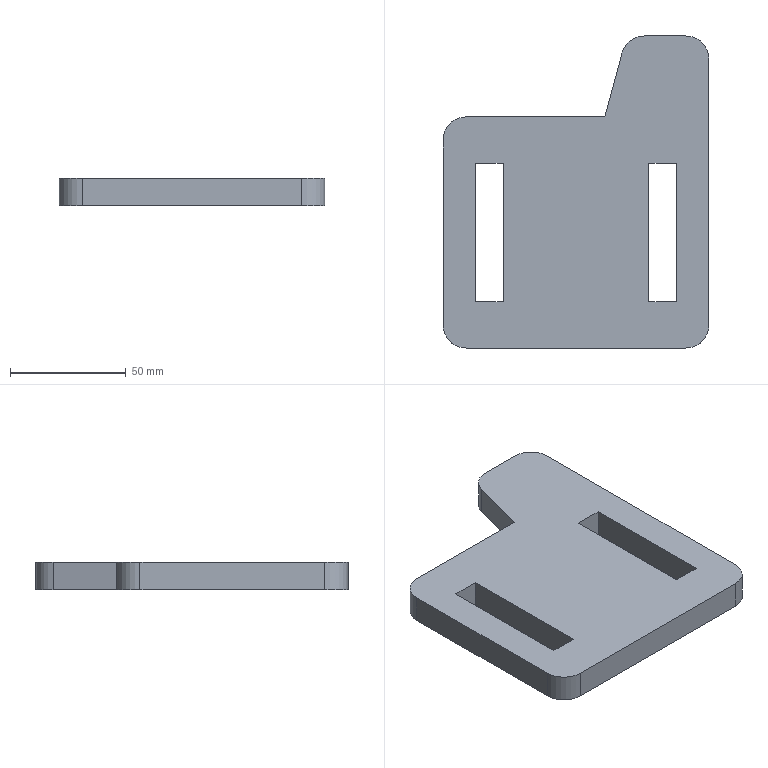Part | SolidWorks | features FlatPattern 1, SMBaseFlange 1, SheetMetal 1 | 1 solid | 21 faces | box 115 x 135 x 12 mm | volume 136485 mm3 | plane 16 | cylinder 5 | commonest cylinder face diameters 20 x5
STEP:
#1=CARTESIAN_POINT('',(3.778,-205.509,0.));
#2=VERTEX_POINT('',#1);
#3=CARTESIAN_POINT('',(-56.222,-205.509,0.));
#4=VERTEX_POINT('',#3);
#5=CARTESIAN_POINT('',(3.778,-205.509,0.));
#6=DIRECTION('',(-1.,0.,0.));
#7=VECTOR('',#6,1000.);
#8=LINE('',#5,#7);
#9=EDGE_CURVE('',#2,#4,#8,.T.);
#10=ORIENTED_EDGE('',*,*,#9,.F.);
#11=CARTESIAN_POINT('',(3.778,-205.509,-12.));
#12=VERTEX_POINT('',#11);
#13=CARTESIAN_POINT('',(3.778,-205.509,-12.));
#14=DIRECTION('',(0.,0.,1.));
#15=VECTOR('',#14,1000.);
#16=LINE('',#13,#15);
#17=EDGE_CURVE('',#12,#2,#16,.T.);
#18=ORIENTED_EDGE('',*,*,#17,.F.);
#19=CARTESIAN_POINT('',(-56.222,-205.509,-12.));
#20=VERTEX_POINT('',#19);
#21=CARTESIAN_POINT('',(3.778,-205.509,-12.));
#22=DIRECTION('',(-1.,0.,0.));
#23=VECTOR('',#22,1000.);
#24=LINE('',#21,#23);
#25=EDGE_CURVE('',#12,#20,#24,.T.);
#26=ORIENTED_EDGE('',*,*,#25,.T.);
#27=CARTESIAN_POINT('',(-56.222,-205.509,-12.));
#28=DIRECTION('',(0.,0.,1.));
#29=VECTOR('',#28,1000.);
#30=LINE('',#27,#29);
#31=EDGE_CURVE('',#20,#4,#30,.T.);
#32=ORIENTED_EDGE('',*,*,#31,.T.);
#33=EDGE_LOOP('',(#10,#18,#26,#32));
#34=FACE_OUTER_BOUND('',#33,.T.);
#35=CARTESIAN_POINT('',(3.778,-205.509,-12.));
#36=DIRECTION('',(0.,1.,0.));
#37=DIRECTION('',(0.,0.,1.));
#38=AXIS2_PLACEMENT_3D('',#35,#36,#37);
#39=PLANE('',#38);
#40=ADVANCED_FACE('',(#34),#39,.T.);
#41=CARTESIAN_POINT('',(11.17,-177.921,0.));
#42=VERTEX_POINT('',#41);
#43=CARTESIAN_POINT('',(11.17,-177.921,0.));
#44=DIRECTION('',(-0.2588,-0.9659,0.));
#45=VECTOR('',#44,1000.);
#46=LINE('',#43,#45);
#47=EDGE_CURVE('',#42,#2,#46,.T.);
#48=ORIENTED_EDGE('',*,*,#47,.F.);
#49=CARTESIAN_POINT('',(11.17,-177.921,-12.));
#50=VERTEX_POINT('',#49);
#51=CARTESIAN_POINT('',(11.17,-177.921,-12.));
#52=DIRECTION('',(0.,0.,1.));
#53=VECTOR('',#52,1000.);
#54=LINE('',#51,#53);
#55=EDGE_CURVE('',#50,#42,#54,.T.);
#56=ORIENTED_EDGE('',*,*,#55,.F.);
#57=CARTESIAN_POINT('',(11.17,-177.921,-12.));
#58=DIRECTION('',(-0.2588,-0.9659,0.));
#59=VECTOR('',#58,1000.);
#60=LINE('',#57,#59);
#61=EDGE_CURVE('',#50,#12,#60,.T.);
#62=ORIENTED_EDGE('',*,*,#61,.T.);
#63=ORIENTED_EDGE('',*,*,#17,.T.);
#64=EDGE_LOOP('',(#48,#56,#62,#63));
#65=FACE_OUTER_BOUND('',#64,.T.);
#66=CARTESIAN_POINT('',(11.17,-177.921,-12.));
#67=DIRECTION('',(-0.9659,0.2588,0.));
#68=DIRECTION('',(-0.2588,-0.9659,0.));
#69=AXIS2_PLACEMENT_3D('',#66,#67,#68);
#70=PLANE('',#69);
#71=ADVANCED_FACE('',(#65),#70,.T.);
#72=CARTESIAN_POINT('',(20.829,-170.509,0.));
#73=VERTEX_POINT('',#72);
#74=CARTESIAN_POINT('',(20.829,-180.509,0.));
#75=DIRECTION('',(0.,0.,1.));
#76=DIRECTION('',(1.,0.,0.));
#77=AXIS2_PLACEMENT_3D('',#74,#75,#76);
#78=CIRCLE('',#77,10.);
#79=EDGE_CURVE('',#73,#42,#78,.T.);
#80=ORIENTED_EDGE('',*,*,#79,.F.);
#81=CARTESIAN_POINT('',(20.829,-170.509,-12.));
#82=VERTEX_POINT('',#81);
#83=CARTESIAN_POINT('',(20.829,-170.509,-12.));
#84=DIRECTION('',(0.,0.,1.));
#85=VECTOR('',#84,1000.);
#86=LINE('',#83,#85);
#87=EDGE_CURVE('',#82,#73,#86,.T.);
#88=ORIENTED_EDGE('',*,*,#87,.F.);
#89=CARTESIAN_POINT('',(20.829,-180.509,-12.));
#90=DIRECTION('',(0.,0.,1.));
#91=DIRECTION('',(1.,0.,0.));
#92=AXIS2_PLACEMENT_3D('',#89,#90,#91);
#93=CIRCLE('',#92,10.);
#94=EDGE_CURVE('',#82,#50,#93,.T.);
#95=ORIENTED_EDGE('',*,*,#94,.T.);
#96=ORIENTED_EDGE('',*,*,#55,.T.);
#97=EDGE_LOOP('',(#80,#88,#95,#96));
#98=FACE_OUTER_BOUND('',#97,.T.);
#99=CARTESIAN_POINT('',(20.829,-180.509,-12.));
#100=DIRECTION('',(0.,0.,1.));
#101=DIRECTION('',(1.,0.,0.));
#102=AXIS2_PLACEMENT_3D('',#99,#100,#101);
#103=CYLINDRICAL_SURFACE('',#102,10.);
#104=ADVANCED_FACE('',(#98),#103,.T.);
#105=CARTESIAN_POINT('',(38.778,-170.509,0.));
#106=VERTEX_POINT('',#105);
#107=CARTESIAN_POINT('',(20.829,-170.509,0.));
#108=DIRECTION('',(-1.,0.,0.));
#109=VECTOR('',#108,1000.);
#110=LINE('',#107,#109);
#111=EDGE_CURVE('',#106,#73,#110,.T.);
#112=ORIENTED_EDGE('',*,*,#111,.F.);
#113=CARTESIAN_POINT('',(38.778,-170.509,-12.));
#114=VERTEX_POINT('',#113);
#115=CARTESIAN_POINT('',(38.778,-170.509,-12.));
#116=DIRECTION('',(0.,0.,1.));
#117=VECTOR('',#116,1000.);
#118=LINE('',#115,#117);
#119=EDGE_CURVE('',#114,#106,#118,.T.);
#120=ORIENTED_EDGE('',*,*,#119,.F.);
#121=CARTESIAN_POINT('',(20.829,-170.509,-12.));
#122=DIRECTION('',(-1.,0.,0.));
#123=VECTOR('',#122,1000.);
#124=LINE('',#121,#123);
#125=EDGE_CURVE('',#114,#82,#124,.T.);
#126=ORIENTED_EDGE('',*,*,#125,.T.);
#127=ORIENTED_EDGE('',*,*,#87,.T.);
#128=EDGE_LOOP('',(#112,#120,#126,#127));
#129=FACE_OUTER_BOUND('',#128,.T.);
#130=CARTESIAN_POINT('',(20.829,-170.509,-12.));
#131=DIRECTION('',(0.,1.,0.));
#132=DIRECTION('',(-1.,0.,0.));
#133=AXIS2_PLACEMENT_3D('',#130,#131,#132);
#134=PLANE('',#133);
#135=ADVANCED_FACE('',(#129),#134,.T.);
#136=CARTESIAN_POINT('',(48.778,-180.509,0.));
#137=VERTEX_POINT('',#136);
#138=CARTESIAN_POINT('',(38.778,-180.509,0.));
#139=DIRECTION('',(0.,0.,1.));
#140=DIRECTION('',(-1.,0.,0.));
#141=AXIS2_PLACEMENT_3D('',#138,#139,#140);
#142=CIRCLE('',#141,10.);
#143=EDGE_CURVE('',#137,#106,#142,.T.);
#144=ORIENTED_EDGE('',*,*,#143,.F.);
#145=CARTESIAN_POINT('',(48.778,-180.509,-12.));
#146=VERTEX_POINT('',#145);
#147=CARTESIAN_POINT('',(48.778,-180.509,-12.));
#148=DIRECTION('',(0.,0.,1.));
#149=VECTOR('',#148,1000.);
#150=LINE('',#147,#149);
#151=EDGE_CURVE('',#146,#137,#150,.T.);
#152=ORIENTED_EDGE('',*,*,#151,.F.);
#153=CARTESIAN_POINT('',(38.778,-180.509,-12.));
#154=DIRECTION('',(0.,0.,1.));
#155=DIRECTION('',(-1.,0.,0.));
#156=AXIS2_PLACEMENT_3D('',#153,#154,#155);
#157=CIRCLE('',#156,10.);
#158=EDGE_CURVE('',#146,#114,#157,.T.);
#159=ORIENTED_EDGE('',*,*,#158,.T.);
#160=ORIENTED_EDGE('',*,*,#119,.T.);
#161=EDGE_LOOP('',(#144,#152,#159,#160));
#162=FACE_OUTER_BOUND('',#161,.T.);
#163=CARTESIAN_POINT('',(38.778,-180.509,-12.));
#164=DIRECTION('',(0.,0.,1.));
#165=DIRECTION('',(1.,0.,0.));
#166=AXIS2_PLACEMENT_3D('',#163,#164,#165);
#167=CYLINDRICAL_SURFACE('',#166,10.);
#168=ADVANCED_FACE('',(#162),#167,.T.);
#169=CARTESIAN_POINT('',(48.778,-295.509,0.));
#170=VERTEX_POINT('',#169);
#171=CARTESIAN_POINT('',(48.778,-180.509,0.));
#172=DIRECTION('',(0.,1.,0.));
#173=VECTOR('',#172,1000.);
#174=LINE('',#171,#173);
#175=EDGE_CURVE('',#170,#137,#174,.T.);
#176=ORIENTED_EDGE('',*,*,#175,.F.);
#177=CARTESIAN_POINT('',(48.778,-295.509,-12.));
#178=VERTEX_POINT('',#177);
#179=CARTESIAN_POINT('',(48.778,-295.509,-12.));
#180=DIRECTION('',(0.,0.,1.));
#181=VECTOR('',#180,1000.);
#182=LINE('',#179,#181);
#183=EDGE_CURVE('',#178,#170,#182,.T.);
#184=ORIENTED_EDGE('',*,*,#183,.F.);
#185=CARTESIAN_POINT('',(48.778,-180.509,-12.));
#186=DIRECTION('',(0.,1.,0.));
#187=VECTOR('',#186,1000.);
#188=LINE('',#185,#187);
#189=EDGE_CURVE('',#178,#146,#188,.T.);
#190=ORIENTED_EDGE('',*,*,#189,.T.);
#191=ORIENTED_EDGE('',*,*,#151,.T.);
#192=EDGE_LOOP('',(#176,#184,#190,#191));
#193=FACE_OUTER_BOUND('',#192,.T.);
#194=CARTESIAN_POINT('',(48.778,-180.509,-12.));
#195=DIRECTION('',(1.,0.,0.));
#196=DIRECTION('',(0.,1.,0.));
#197=AXIS2_PLACEMENT_3D('',#194,#195,#196);
#198=PLANE('',#197);
#199=ADVANCED_FACE('',(#193),#198,.T.);
#200=CARTESIAN_POINT('',(38.778,-305.509,0.));
#201=VERTEX_POINT('',#200);
#202=CARTESIAN_POINT('',(38.778,-295.509,0.));
#203=DIRECTION('',(0.,0.,1.));
#204=DIRECTION('',(-1.,0.,0.));
#205=AXIS2_PLACEMENT_3D('',#202,#203,#204);
#206=CIRCLE('',#205,10.);
#207=EDGE_CURVE('',#201,#170,#206,.T.);
#208=ORIENTED_EDGE('',*,*,#207,.F.);
#209=CARTESIAN_POINT('',(38.778,-305.509,-12.));
#210=VERTEX_POINT('',#209);
#211=CARTESIAN_POINT('',(38.778,-305.509,-12.));
#212=DIRECTION('',(0.,0.,1.));
#213=VECTOR('',#212,1000.);
#214=LINE('',#211,#213);
#215=EDGE_CURVE('',#210,#201,#214,.T.);
#216=ORIENTED_EDGE('',*,*,#215,.F.);
#217=CARTESIAN_POINT('',(38.778,-295.509,-12.));
#218=DIRECTION('',(0.,0.,1.));
#219=DIRECTION('',(-1.,0.,0.));
#220=AXIS2_PLACEMENT_3D('',#217,#218,#219);
#221=CIRCLE('',#220,10.);
#222=EDGE_CURVE('',#210,#178,#221,.T.);
#223=ORIENTED_EDGE('',*,*,#222,.T.);
#224=ORIENTED_EDGE('',*,*,#183,.T.);
#225=EDGE_LOOP('',(#208,#216,#223,#224));
#226=FACE_OUTER_BOUND('',#225,.T.);
#227=CARTESIAN_POINT('',(38.778,-295.509,-12.));
#228=DIRECTION('',(0.,0.,1.));
#229=DIRECTION('',(1.,0.,0.));
#230=AXIS2_PLACEMENT_3D('',#227,#228,#229);
#231=CYLINDRICAL_SURFACE('',#230,10.);
#232=ADVANCED_FACE('',(#226),#231,.T.);
#233=CARTESIAN_POINT('',(-56.222,-305.509,0.));
#234=VERTEX_POINT('',#233);
#235=CARTESIAN_POINT('',(-56.222,-305.509,0.));
#236=DIRECTION('',(1.,0.,0.));
#237=VECTOR('',#236,1000.);
#238=LINE('',#235,#237);
#239=EDGE_CURVE('',#234,#201,#238,.T.);
#240=ORIENTED_EDGE('',*,*,#239,.F.);
#241=CARTESIAN_POINT('',(-56.222,-305.509,-12.));
#242=VERTEX_POINT('',#241);
#243=CARTESIAN_POINT('',(-56.222,-305.509,-12.));
#244=DIRECTION('',(0.,0.,1.));
#245=VECTOR('',#244,1000.);
#246=LINE('',#243,#245);
#247=EDGE_CURVE('',#242,#234,#246,.T.);
#248=ORIENTED_EDGE('',*,*,#247,.F.);
#249=CARTESIAN_POINT('',(-56.222,-305.509,-12.));
#250=DIRECTION('',(1.,0.,0.));
#251=VECTOR('',#250,1000.);
#252=LINE('',#249,#251);
#253=EDGE_CURVE('',#242,#210,#252,.T.);
#254=ORIENTED_EDGE('',*,*,#253,.T.);
#255=ORIENTED_EDGE('',*,*,#215,.T.);
#256=EDGE_LOOP('',(#240,#248,#254,#255));
#257=FACE_OUTER_BOUND('',#256,.T.);
#258=CARTESIAN_POINT('',(-56.222,-305.509,-12.));
#259=DIRECTION('',(0.,-1.,0.));
#260=DIRECTION('',(0.,0.,-1.));
#261=AXIS2_PLACEMENT_3D('',#258,#259,#260);
#262=PLANE('',#261);
#263=ADVANCED_FACE('',(#257),#262,.T.);
#264=CARTESIAN_POINT('',(-66.222,-295.509,0.));
#265=VERTEX_POINT('',#264);
#266=CARTESIAN_POINT('',(-56.222,-295.509,0.));
#267=DIRECTION('',(0.,0.,1.));
#268=DIRECTION('',(1.,0.,0.));
#269=AXIS2_PLACEMENT_3D('',#266,#267,#268);
#270=CIRCLE('',#269,10.);
#271=EDGE_CURVE('',#265,#234,#270,.T.);
#272=ORIENTED_EDGE('',*,*,#271,.F.);
#273=CARTESIAN_POINT('',(-66.222,-295.509,-12.));
#274=VERTEX_POINT('',#273);
#275=CARTESIAN_POINT('',(-66.222,-295.509,-12.));
#276=DIRECTION('',(0.,0.,1.));
#277=VECTOR('',#276,1000.);
#278=LINE('',#275,#277);
#279=EDGE_CURVE('',#274,#265,#278,.T.);
#280=ORIENTED_EDGE('',*,*,#279,.F.);
#281=CARTESIAN_POINT('',(-56.222,-295.509,-12.));
#282=DIRECTION('',(0.,0.,1.));
#283=DIRECTION('',(1.,0.,0.));
#284=AXIS2_PLACEMENT_3D('',#281,#282,#283);
#285=CIRCLE('',#284,10.);
#286=EDGE_CURVE('',#274,#242,#285,.T.);
#287=ORIENTED_EDGE('',*,*,#286,.T.);
#288=ORIENTED_EDGE('',*,*,#247,.T.);
#289=EDGE_LOOP('',(#272,#280,#287,#288));
#290=FACE_OUTER_BOUND('',#289,.T.);
#291=CARTESIAN_POINT('',(-56.222,-295.509,-12.));
#292=DIRECTION('',(0.,0.,1.));
#293=DIRECTION('',(1.,0.,0.));
#294=AXIS2_PLACEMENT_3D('',#291,#292,#293);
#295=CYLINDRICAL_SURFACE('',#294,10.);
#296=ADVANCED_FACE('',(#290),#295,.T.);
#297=CARTESIAN_POINT('',(-66.222,-215.509,0.));
#298=VERTEX_POINT('',#297);
#299=CARTESIAN_POINT('',(-66.222,-215.509,0.));
#300=DIRECTION('',(0.,-1.,0.));
#301=VECTOR('',#300,1000.);
#302=LINE('',#299,#301);
#303=EDGE_CURVE('',#298,#265,#302,.T.);
#304=ORIENTED_EDGE('',*,*,#303,.F.);
#305=CARTESIAN_POINT('',(-66.222,-215.509,-12.));
#306=VERTEX_POINT('',#305);
#307=CARTESIAN_POINT('',(-66.222,-215.509,-12.));
#308=DIRECTION('',(0.,0.,1.));
#309=VECTOR('',#308,1000.);
#310=LINE('',#307,#309);
#311=EDGE_CURVE('',#306,#298,#310,.T.);
#312=ORIENTED_EDGE('',*,*,#311,.F.);
#313=CARTESIAN_POINT('',(-66.222,-215.509,-12.));
#314=DIRECTION('',(0.,-1.,0.));
#315=VECTOR('',#314,1000.);
#316=LINE('',#313,#315);
#317=EDGE_CURVE('',#306,#274,#316,.T.);
#318=ORIENTED_EDGE('',*,*,#317,.T.);
#319=ORIENTED_EDGE('',*,*,#279,.T.);
#320=EDGE_LOOP('',(#304,#312,#318,#319));
#321=FACE_OUTER_BOUND('',#320,.T.);
#322=CARTESIAN_POINT('',(-66.222,-215.509,-12.));
#323=DIRECTION('',(-1.,0.,0.));
#324=DIRECTION('',(0.,-1.,0.));
#325=AXIS2_PLACEMENT_3D('',#322,#323,#324);
#326=PLANE('',#325);
#327=ADVANCED_FACE('',(#321),#326,.T.);
#328=CARTESIAN_POINT('',(-56.222,-215.509,0.));
#329=DIRECTION('',(0.,0.,1.));
#330=DIRECTION('',(1.,0.,0.));
#331=AXIS2_PLACEMENT_3D('',#328,#329,#330);
#332=CIRCLE('',#331,10.);
#333=EDGE_CURVE('',#4,#298,#332,.T.);
#334=ORIENTED_EDGE('',*,*,#333,.F.);
#335=ORIENTED_EDGE('',*,*,#31,.F.);
#336=CARTESIAN_POINT('',(-56.222,-215.509,-12.));
#337=DIRECTION('',(0.,0.,1.));
#338=DIRECTION('',(1.,0.,0.));
#339=AXIS2_PLACEMENT_3D('',#336,#337,#338);
#340=CIRCLE('',#339,10.);
#341=EDGE_CURVE('',#20,#306,#340,.T.);
#342=ORIENTED_EDGE('',*,*,#341,.T.);
#343=ORIENTED_EDGE('',*,*,#311,.T.);
#344=EDGE_LOOP('',(#334,#335,#342,#343));
#345=FACE_OUTER_BOUND('',#344,.T.);
#346=CARTESIAN_POINT('',(-56.222,-215.509,-12.));
#347=DIRECTION('',(0.,0.,1.));
#348=DIRECTION('',(1.,0.,0.));
#349=AXIS2_PLACEMENT_3D('',#346,#347,#348);
#350=CYLINDRICAL_SURFACE('',#349,10.);
#351=ADVANCED_FACE('',(#345),#350,.T.);
#352=CARTESIAN_POINT('',(-40.222,-225.509,-12.));
#353=VERTEX_POINT('',#352);
#354=CARTESIAN_POINT('',(-52.222,-225.509,-12.));
#355=VERTEX_POINT('',#354);
#356=CARTESIAN_POINT('',(-52.222,-225.509,-12.));
#357=DIRECTION('',(-1.,0.,0.));
#358=VECTOR('',#357,1000.);
#359=LINE('',#356,#358);
#360=EDGE_CURVE('',#353,#355,#359,.T.);
#361=ORIENTED_EDGE('',*,*,#360,.T.);
#362=CARTESIAN_POINT('',(-52.222,-285.509,-12.));
#363=VERTEX_POINT('',#362);
#364=CARTESIAN_POINT('',(-52.222,-225.509,-12.));
#365=DIRECTION('',(0.,-1.,0.));
#366=VECTOR('',#365,1000.);
#367=LINE('',#364,#366);
#368=EDGE_CURVE('',#355,#363,#367,.T.);
#369=ORIENTED_EDGE('',*,*,#368,.T.);
#370=CARTESIAN_POINT('',(-40.222,-285.509,-12.));
#371=VERTEX_POINT('',#370);
#372=CARTESIAN_POINT('',(-52.222,-285.509,-12.));
#373=DIRECTION('',(1.,0.,0.));
#374=VECTOR('',#373,1000.);
#375=LINE('',#372,#374);
#376=EDGE_CURVE('',#363,#371,#375,.T.);
#377=ORIENTED_EDGE('',*,*,#376,.T.);
#378=CARTESIAN_POINT('',(-40.222,-225.509,-12.));
#379=DIRECTION('',(0.,1.,0.));
#380=VECTOR('',#379,1000.);
#381=LINE('',#378,#380);
#382=EDGE_CURVE('',#371,#353,#381,.T.);
#383=ORIENTED_EDGE('',*,*,#382,.T.);
#384=EDGE_LOOP('',(#361,#369,#377,#383));
#385=FACE_BOUND('',#384,.T.);
#386=CARTESIAN_POINT('',(34.778,-225.509,-12.));
#387=VERTEX_POINT('',#386);
#388=CARTESIAN_POINT('',(22.778,-225.509,-12.));
#389=VERTEX_POINT('',#388);
#390=CARTESIAN_POINT('',(22.778,-225.509,-12.));
#391=DIRECTION('',(-1.,0.,0.));
#392=VECTOR('',#391,1000.);
#393=LINE('',#390,#392);
#394=EDGE_CURVE('',#387,#389,#393,.T.);
#395=ORIENTED_EDGE('',*,*,#394,.T.);
#396=CARTESIAN_POINT('',(22.778,-285.509,-12.));
#397=VERTEX_POINT('',#396);
#398=CARTESIAN_POINT('',(22.778,-225.509,-12.));
#399=DIRECTION('',(0.,-1.,0.));
#400=VECTOR('',#399,1000.);
#401=LINE('',#398,#400);
#402=EDGE_CURVE('',#389,#397,#401,.T.);
#403=ORIENTED_EDGE('',*,*,#402,.T.);
#404=CARTESIAN_POINT('',(34.778,-285.509,-12.));
#405=VERTEX_POINT('',#404);
#406=CARTESIAN_POINT('',(22.778,-285.509,-12.));
#407=DIRECTION('',(1.,0.,0.));
#408=VECTOR('',#407,1000.);
#409=LINE('',#406,#408);
#410=EDGE_CURVE('',#397,#405,#409,.T.);
#411=ORIENTED_EDGE('',*,*,#410,.T.);
#412=CARTESIAN_POINT('',(34.778,-225.509,-12.));
#413=DIRECTION('',(0.,1.,0.));
#414=VECTOR('',#413,1000.);
#415=LINE('',#412,#414);
#416=EDGE_CURVE('',#405,#387,#415,.T.);
#417=ORIENTED_EDGE('',*,*,#416,.T.);
#418=EDGE_LOOP('',(#395,#403,#411,#417));
#419=FACE_BOUND('',#418,.T.);
#420=ORIENTED_EDGE('',*,*,#25,.F.);
#421=ORIENTED_EDGE('',*,*,#61,.F.);
#422=ORIENTED_EDGE('',*,*,#94,.F.);
#423=ORIENTED_EDGE('',*,*,#125,.F.);
#424=ORIENTED_EDGE('',*,*,#158,.F.);
#425=ORIENTED_EDGE('',*,*,#189,.F.);
#426=ORIENTED_EDGE('',*,*,#222,.F.);
#427=ORIENTED_EDGE('',*,*,#253,.F.);
#428=ORIENTED_EDGE('',*,*,#286,.F.);
#429=ORIENTED_EDGE('',*,*,#317,.F.);
#430=ORIENTED_EDGE('',*,*,#341,.F.);
#431=EDGE_LOOP('',(#420,#421,#422,#423,#424,#425,#426,#427,#428,#429,#430));
#432=FACE_OUTER_BOUND('',#431,.T.);
#433=CARTESIAN_POINT('',(-56.222,-215.509,-12.));
#434=DIRECTION('',(0.,0.,1.));
#435=DIRECTION('',(1.,0.,0.));
#436=AXIS2_PLACEMENT_3D('',#433,#434,#435);
#437=PLANE('',#436);
#438=ADVANCED_FACE('',(#385,#419,#432),#437,.F.);
#439=CARTESIAN_POINT('',(-52.222,-225.509,0.));
#440=VERTEX_POINT('',#439);
#441=CARTESIAN_POINT('',(-52.222,-285.509,0.));
#442=VERTEX_POINT('',#441);
#443=CARTESIAN_POINT('',(-52.222,-225.509,0.));
#444=DIRECTION('',(0.,-1.,0.));
#445=VECTOR('',#444,1000.);
#446=LINE('',#443,#445);
#447=EDGE_CURVE('',#440,#442,#446,.T.);
#448=ORIENTED_EDGE('',*,*,#447,.F.);
#449=CARTESIAN_POINT('',(-40.222,-225.509,0.));
#450=VERTEX_POINT('',#449);
#451=CARTESIAN_POINT('',(-52.222,-225.509,0.));
#452=DIRECTION('',(-1.,0.,0.));
#453=VECTOR('',#452,1000.);
#454=LINE('',#451,#453);
#455=EDGE_CURVE('',#450,#440,#454,.T.);
#456=ORIENTED_EDGE('',*,*,#455,.F.);
#457=CARTESIAN_POINT('',(-40.222,-285.509,0.));
#458=VERTEX_POINT('',#457);
#459=CARTESIAN_POINT('',(-40.222,-225.509,0.));
#460=DIRECTION('',(0.,1.,0.));
#461=VECTOR('',#460,1000.);
#462=LINE('',#459,#461);
#463=EDGE_CURVE('',#458,#450,#462,.T.);
#464=ORIENTED_EDGE('',*,*,#463,.F.);
#465=CARTESIAN_POINT('',(-52.222,-285.509,0.));
#466=DIRECTION('',(1.,0.,0.));
#467=VECTOR('',#466,1000.);
#468=LINE('',#465,#467);
#469=EDGE_CURVE('',#442,#458,#468,.T.);
#470=ORIENTED_EDGE('',*,*,#469,.F.);
#471=EDGE_LOOP('',(#448,#456,#464,#470));
#472=FACE_BOUND('',#471,.T.);
#473=CARTESIAN_POINT('',(22.778,-225.509,0.));
#474=VERTEX_POINT('',#473);
#475=CARTESIAN_POINT('',(22.778,-285.509,0.));
#476=VERTEX_POINT('',#475);
#477=CARTESIAN_POINT('',(22.778,-225.509,0.));
#478=DIRECTION('',(0.,-1.,0.));
#479=VECTOR('',#478,1000.);
#480=LINE('',#477,#479);
#481=EDGE_CURVE('',#474,#476,#480,.T.);
#482=ORIENTED_EDGE('',*,*,#481,.F.);
#483=CARTESIAN_POINT('',(34.778,-225.509,0.));
#484=VERTEX_POINT('',#483);
#485=CARTESIAN_POINT('',(22.778,-225.509,0.));
#486=DIRECTION('',(-1.,0.,0.));
#487=VECTOR('',#486,1000.);
#488=LINE('',#485,#487);
#489=EDGE_CURVE('',#484,#474,#488,.T.);
#490=ORIENTED_EDGE('',*,*,#489,.F.);
#491=CARTESIAN_POINT('',(34.778,-285.509,0.));
#492=VERTEX_POINT('',#491);
#493=CARTESIAN_POINT('',(34.778,-225.509,0.));
#494=DIRECTION('',(0.,1.,0.));
#495=VECTOR('',#494,1000.);
#496=LINE('',#493,#495);
#497=EDGE_CURVE('',#492,#484,#496,.T.);
#498=ORIENTED_EDGE('',*,*,#497,.F.);
#499=CARTESIAN_POINT('',(22.778,-285.509,0.));
#500=DIRECTION('',(1.,0.,0.));
#501=VECTOR('',#500,1000.);
#502=LINE('',#499,#501);
#503=EDGE_CURVE('',#476,#492,#502,.T.);
#504=ORIENTED_EDGE('',*,*,#503,.F.);
#505=EDGE_LOOP('',(#482,#490,#498,#504));
#506=FACE_BOUND('',#505,.T.);
#507=ORIENTED_EDGE('',*,*,#9,.T.);
#508=ORIENTED_EDGE('',*,*,#333,.T.);
#509=ORIENTED_EDGE('',*,*,#303,.T.);
#510=ORIENTED_EDGE('',*,*,#271,.T.);
#511=ORIENTED_EDGE('',*,*,#239,.T.);
#512=ORIENTED_EDGE('',*,*,#207,.T.);
#513=ORIENTED_EDGE('',*,*,#175,.T.);
#514=ORIENTED_EDGE('',*,*,#143,.T.);
#515=ORIENTED_EDGE('',*,*,#111,.T.);
#516=ORIENTED_EDGE('',*,*,#79,.T.);
#517=ORIENTED_EDGE('',*,*,#47,.T.);
#518=EDGE_LOOP('',(#507,#508,#509,#510,#511,#512,#513,#514,#515,#516,#517));
#519=FACE_OUTER_BOUND('',#518,.T.);
#520=CARTESIAN_POINT('',(-56.222,-215.509,0.));
#521=DIRECTION('',(0.,0.,1.));
#522=DIRECTION('',(1.,0.,0.));
#523=AXIS2_PLACEMENT_3D('',#520,#521,#522);
#524=PLANE('',#523);
#525=ADVANCED_FACE('',(#472,#506,#519),#524,.T.);
#526=ORIENTED_EDGE('',*,*,#481,.T.);
#527=CARTESIAN_POINT('',(22.778,-285.509,-12.));
#528=DIRECTION('',(0.,0.,1.));
#529=VECTOR('',#528,1000.);
#530=LINE('',#527,#529);
#531=EDGE_CURVE('',#397,#476,#530,.T.);
#532=ORIENTED_EDGE('',*,*,#531,.F.);
#533=ORIENTED_EDGE('',*,*,#402,.F.);
#534=CARTESIAN_POINT('',(22.778,-225.509,-12.));
#535=DIRECTION('',(0.,0.,1.));
#536=VECTOR('',#535,1000.);
#537=LINE('',#534,#536);
#538=EDGE_CURVE('',#389,#474,#537,.T.);
#539=ORIENTED_EDGE('',*,*,#538,.T.);
#540=EDGE_LOOP('',(#526,#532,#533,#539));
#541=FACE_OUTER_BOUND('',#540,.T.);
#542=CARTESIAN_POINT('',(22.778,-225.509,-12.));
#543=DIRECTION('',(-1.,0.,0.));
#544=DIRECTION('',(0.,-1.,0.));
#545=AXIS2_PLACEMENT_3D('',#542,#543,#544);
#546=PLANE('',#545);
#547=ADVANCED_FACE('',(#541),#546,.F.);
#548=ORIENTED_EDGE('',*,*,#489,.T.);
#549=ORIENTED_EDGE('',*,*,#538,.F.);
#550=ORIENTED_EDGE('',*,*,#394,.F.);
#551=CARTESIAN_POINT('',(34.778,-225.509,-12.));
#552=DIRECTION('',(0.,0.,1.));
#553=VECTOR('',#552,1000.);
#554=LINE('',#551,#553);
#555=EDGE_CURVE('',#387,#484,#554,.T.);
#556=ORIENTED_EDGE('',*,*,#555,.T.);
#557=EDGE_LOOP('',(#548,#549,#550,#556));
#558=FACE_OUTER_BOUND('',#557,.T.);
#559=CARTESIAN_POINT('',(22.778,-225.509,-12.));
#560=DIRECTION('',(0.,1.,0.));
#561=DIRECTION('',(0.,0.,1.));
#562=AXIS2_PLACEMENT_3D('',#559,#560,#561);
#563=PLANE('',#562);
#564=ADVANCED_FACE('',(#558),#563,.F.);
#565=ORIENTED_EDGE('',*,*,#497,.T.);
#566=ORIENTED_EDGE('',*,*,#555,.F.);
#567=ORIENTED_EDGE('',*,*,#416,.F.);
#568=CARTESIAN_POINT('',(34.778,-285.509,-12.));
#569=DIRECTION('',(0.,0.,1.));
#570=VECTOR('',#569,1000.);
#571=LINE('',#568,#570);
#572=EDGE_CURVE('',#405,#492,#571,.T.);
#573=ORIENTED_EDGE('',*,*,#572,.T.);
#574=EDGE_LOOP('',(#565,#566,#567,#573));
#575=FACE_OUTER_BOUND('',#574,.T.);
#576=CARTESIAN_POINT('',(34.778,-225.509,-12.));
#577=DIRECTION('',(1.,0.,0.));
#578=DIRECTION('',(0.,1.,0.));
#579=AXIS2_PLACEMENT_3D('',#576,#577,#578);
#580=PLANE('',#579);
#581=ADVANCED_FACE('',(#575),#580,.F.);
#582=ORIENTED_EDGE('',*,*,#503,.T.);
#583=ORIENTED_EDGE('',*,*,#572,.F.);
#584=ORIENTED_EDGE('',*,*,#410,.F.);
#585=ORIENTED_EDGE('',*,*,#531,.T.);
#586=EDGE_LOOP('',(#582,#583,#584,#585));
#587=FACE_OUTER_BOUND('',#586,.T.);
#588=CARTESIAN_POINT('',(22.778,-285.509,-12.));
#589=DIRECTION('',(0.,-1.,0.));
#590=DIRECTION('',(0.,0.,-1.));
#591=AXIS2_PLACEMENT_3D('',#588,#589,#590);
#592=PLANE('',#591);
#593=ADVANCED_FACE('',(#587),#592,.F.);
#594=ORIENTED_EDGE('',*,*,#447,.T.);
#595=CARTESIAN_POINT('',(-52.222,-285.509,-12.));
#596=DIRECTION('',(0.,0.,1.));
#597=VECTOR('',#596,1000.);
#598=LINE('',#595,#597);
#599=EDGE_CURVE('',#363,#442,#598,.T.);
#600=ORIENTED_EDGE('',*,*,#599,.F.);
#601=ORIENTED_EDGE('',*,*,#368,.F.);
#602=CARTESIAN_POINT('',(-52.222,-225.509,-12.));
#603=DIRECTION('',(0.,0.,1.));
#604=VECTOR('',#603,1000.);
#605=LINE('',#602,#604);
#606=EDGE_CURVE('',#355,#440,#605,.T.);
#607=ORIENTED_EDGE('',*,*,#606,.T.);
#608=EDGE_LOOP('',(#594,#600,#601,#607));
#609=FACE_OUTER_BOUND('',#608,.T.);
#610=CARTESIAN_POINT('',(-52.222,-225.509,-12.));
#611=DIRECTION('',(-1.,0.,0.));
#612=DIRECTION('',(0.,-1.,0.));
#613=AXIS2_PLACEMENT_3D('',#610,#611,#612);
#614=PLANE('',#613);
#615=ADVANCED_FACE('',(#609),#614,.F.);
#616=ORIENTED_EDGE('',*,*,#455,.T.);
#617=ORIENTED_EDGE('',*,*,#606,.F.);
#618=ORIENTED_EDGE('',*,*,#360,.F.);
#619=CARTESIAN_POINT('',(-40.222,-225.509,-12.));
#620=DIRECTION('',(0.,0.,1.));
#621=VECTOR('',#620,1000.);
#622=LINE('',#619,#621);
#623=EDGE_CURVE('',#353,#450,#622,.T.);
#624=ORIENTED_EDGE('',*,*,#623,.T.);
#625=EDGE_LOOP('',(#616,#617,#618,#624));
#626=FACE_OUTER_BOUND('',#625,.T.);
#627=CARTESIAN_POINT('',(-52.222,-225.509,-12.));
#628=DIRECTION('',(0.,1.,0.));
#629=DIRECTION('',(0.,0.,1.));
#630=AXIS2_PLACEMENT_3D('',#627,#628,#629);
#631=PLANE('',#630);
#632=ADVANCED_FACE('',(#626),#631,.F.);
#633=ORIENTED_EDGE('',*,*,#463,.T.);
#634=ORIENTED_EDGE('',*,*,#623,.F.);
#635=ORIENTED_EDGE('',*,*,#382,.F.);
#636=CARTESIAN_POINT('',(-40.222,-285.509,-12.));
#637=DIRECTION('',(0.,0.,1.));
#638=VECTOR('',#637,1000.);
#639=LINE('',#636,#638);
#640=EDGE_CURVE('',#371,#458,#639,.T.);
#641=ORIENTED_EDGE('',*,*,#640,.T.);
#642=EDGE_LOOP('',(#633,#634,#635,#641));
#643=FACE_OUTER_BOUND('',#642,.T.);
#644=CARTESIAN_POINT('',(-40.222,-225.509,-12.));
#645=DIRECTION('',(1.,0.,0.));
#646=DIRECTION('',(0.,1.,0.));
#647=AXIS2_PLACEMENT_3D('',#644,#645,#646);
#648=PLANE('',#647);
#649=ADVANCED_FACE('',(#643),#648,.F.);
#650=ORIENTED_EDGE('',*,*,#469,.T.);
#651=ORIENTED_EDGE('',*,*,#640,.F.);
#652=ORIENTED_EDGE('',*,*,#376,.F.);
#653=ORIENTED_EDGE('',*,*,#599,.T.);
#654=EDGE_LOOP('',(#650,#651,#652,#653));
#655=FACE_OUTER_BOUND('',#654,.T.);
#656=CARTESIAN_POINT('',(-52.222,-285.509,-12.));
#657=DIRECTION('',(0.,-1.,0.));
#658=DIRECTION('',(0.,0.,-1.));
#659=AXIS2_PLACEMENT_3D('',#656,#657,#658);
#660=PLANE('',#659);
#661=ADVANCED_FACE('',(#655),#660,.F.);
#662=CLOSED_SHELL('',(#40,#71,#104,#135,#168,#199,#232,#263,#296,#327,#351,#438,#525,#547,#564,#581,#593,#615,#632,#649,#661));
#663=MANIFOLD_SOLID_BREP('',#662);
#664=CARTESIAN_POINT('',(0.,0.,0.));
#665=DIRECTION('',(0.,0.,1.));
#666=DIRECTION('',(1.,0.,0.));
#667=AXIS2_PLACEMENT_3D('',#664,#665,#666);
#668=(LENGTH_UNIT()NAMED_UNIT(*)SI_UNIT(.MILLI.,.METRE.));
#669=UNCERTAINTY_MEASURE_WITH_UNIT(LENGTH_MEASURE(0.00001),#668,'','');
#670=(NAMED_UNIT(*)PLANE_ANGLE_UNIT()SI_UNIT($,.RADIAN.));
#671=(NAMED_UNIT(*)SI_UNIT($,.STERADIAN.)SOLID_ANGLE_UNIT());
#672=(GEOMETRIC_REPRESENTATION_CONTEXT(3)GLOBAL_UNCERTAINTY_ASSIGNED_CONTEXT((#669))GLOBAL_UNIT_ASSIGNED_CONTEXT((#668,#670,#671))REPRESENTATION_CONTEXT('',''));
#673=ADVANCED_BREP_SHAPE_REPRESENTATION('',(#663,#667),#672);